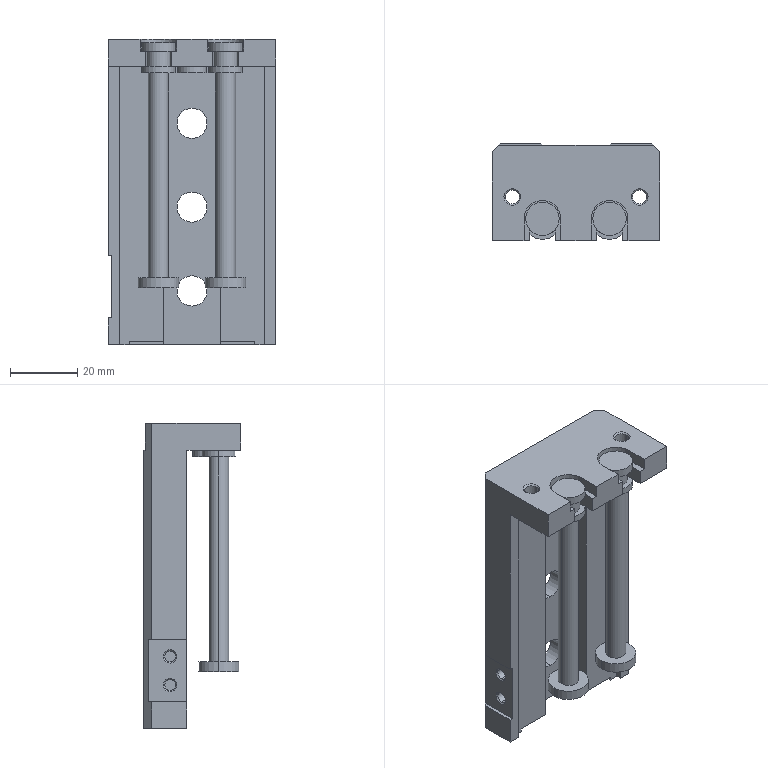Part | SolidWorks | features BaseBody 1 | 1 solid | 176 faces | box 50 x 29 x 91 mm | volume 51453 mm3 | plane 99 | cylinder 61 | cone 16 | commonest cylinder face diameters 3.242 x12 10 x8 9 x6 4 x5 4.134 x4 4.9 x4